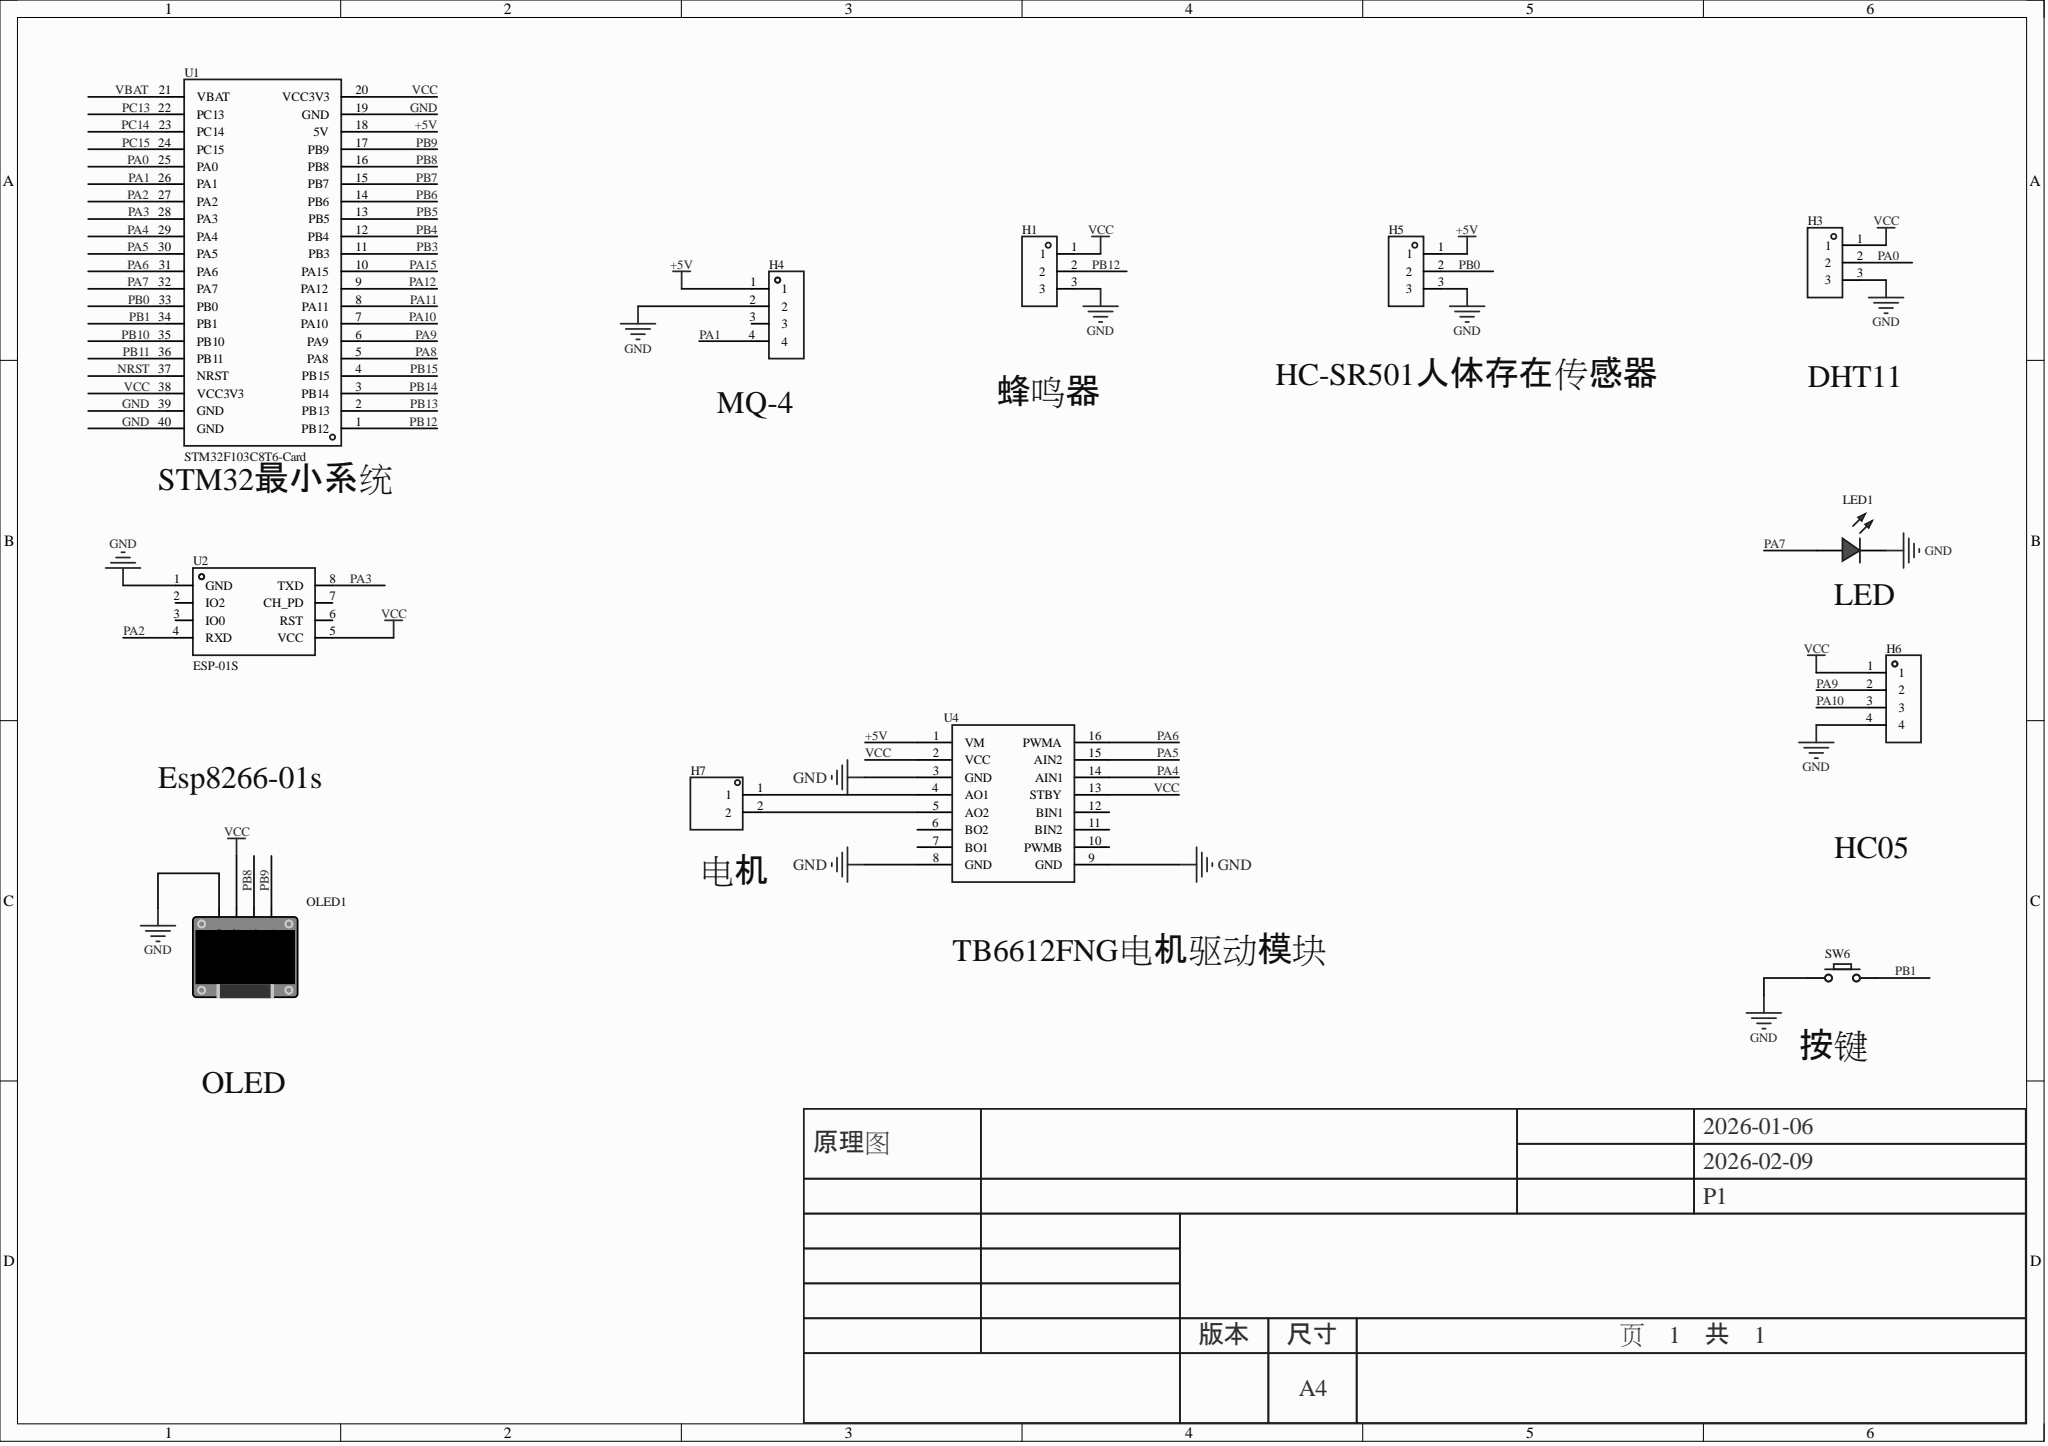Circuit board | Altium Designer | 12 parts | 20 nets
Bill of materials:
Comment,Description,Designator,Footprint,LibRef,Quantity
"","","H1, H3, H5","HDR-TH_3P-P2.54-V-F","HDR-F_2.54_1x3P","3"
"","","H4, H6","HDR-TH_4P-P2.54-V-F","HDR-F_2.54_1x4P","2"
"","","H7","HDR-TH_2P-P2.54-V-M-1","HDR-M_2.54_1x2P","1"
"","","LED1","LED_TH-3mm","LED_TH-R_3mm","1"
"","","OLED1","0.96OLED_4P","0.96OLED模块_4P","1"
"","","SW6","Key_TH_3.5x6x4.3","Key_TH_3.5x6x4.3","1"
"STM32F103C8T6-Card","","U1","CONN-TH_L53.3-W22.9_STM32F103C8T6-CARD","STM32F103C8T6-Card","1"
"ESP-01S","","U2","WIFIM-TH_ESP-01S","ESP-01S_C111009","1"
"","","U4","tb6612","tb6612","1"
Netlist (Protel format):
[
H1
HDR-TH_3P-P2.54-V-F




]
[
H3
HDR-TH_3P-P2.54-V-F




]
[
H4
HDR-TH_4P-P2.54-V-F




]
[
H5
HDR-TH_3P-P2.54-V-F




]
[
H6
HDR-TH_4P-P2.54-V-F




]
[
H7
HDR-TH_2P-P2.54-V-M-1




]
[
LED1
LED_TH-3mm




]
[
OLED1
0.96OLED_4P




]
[
SW6
Key_TH_3.5x6x4.3




]
[
U1
CONN-TH_L53.3-W22.9_STM32F103C8T6-CARD
STM32F103C8T6-Card



]
[
U2
WIFIM-TH_ESP-01S
ESP-01S



]
[
U4
tb6612




]
(
VCC
H1-1
H3-1
H6-1
OLED1-2
U1-20
U1-38
U2-5
U4-2
U4-13
)
(
PB12
H1-2
U1-1
)
(
PB9
OLED1-4
U1-17
)
(
PB8
OLED1-3
U1-16
)
(
PB1
SW6-B
U1-34
)
(
PB0
H5-2
U1-33
)
(
PA10
H6-3
U1-7
)
(
PA9
H6-2
U1-6
)
(
PA7
LED1-1
U1-32
)
(
PA6
U1-31
U4-16
)
(
PA5
U1-30
U4-15
)
(
PA4
U1-29
U4-14
)
(
PA3
U1-28
U2-8
)
(
PA2
U1-27
U2-4
)
(
PA1
H4-4
U1-26
)
(
PA0
H3-2
U1-25
)
(
NetH7_2
H7-2
U4-5
)
(
NetH7_1
H7-1
U4-4
)
(
GND
H1-3
H3-3
H4-2
H5-3
H6-4
LED1-2
OLED1-1
SW6-A
U1-19
U1-39
U1-40
U2-1
U4-3
U4-8
U4-9
)
(
+5V
H4-1
H5-1
U1-18
U4-1
)